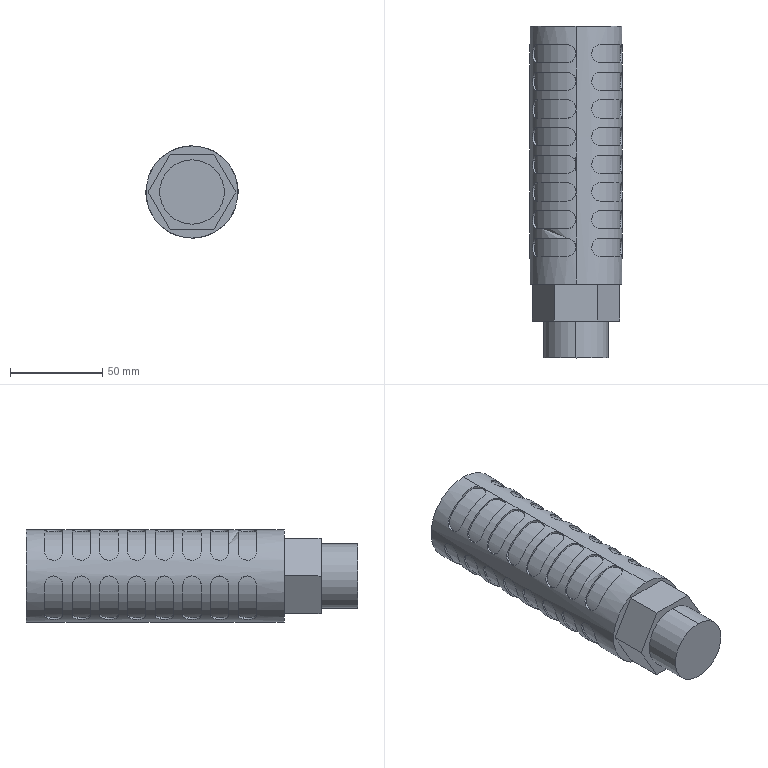Part | STEP file | PN_0013_default | 1 solid | 238 faces | box 50 x 180 x 50 mm | volume 314357 mm3 | cylinder 164 | plane 74 | commonest cylinder face diameters 10 x128 48 x32 35 x2 50 x2